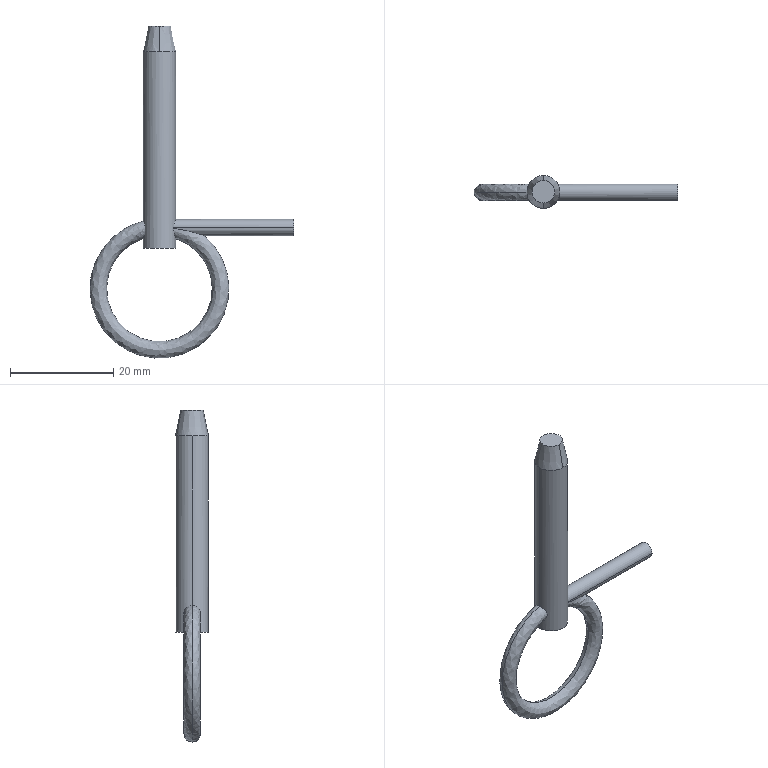Part | SolidWorks | features BaseBody 1 | 1 solid | 11 faces | box 39.425 x 6.35 x 64.25 mm | volume 2028 mm3 | cylinder 4 | plane 3 | cone 2 | spline 2 | commonest cylinder face diameters 3.2 x2 6.35 x2
STEP:
#1=CARTESIAN_POINT('',(3.175,0.,38.));
#2=VERTEX_POINT('',#1);
#3=CARTESIAN_POINT('',(0.,3.175,38.));
#4=VERTEX_POINT('',#3);
#5=CARTESIAN_POINT('',(0.,0.,38.));
#6=DIRECTION('',(0.,0.,1.));
#7=DIRECTION('',(-1.,0.,0.));
#8=AXIS2_PLACEMENT_3D('',#5,#6,#7);
#9=CIRCLE('',#8,3.175);
#10=EDGE_CURVE('',#2,#4,#9,.T.);
#11=ORIENTED_EDGE('',*,*,#10,.F.);
#12=CARTESIAN_POINT('',(3.175,0.,5.6));
#13=VERTEX_POINT('',#12);
#14=CARTESIAN_POINT('',(3.175,0.,38.));
#15=DIRECTION('',(0.,0.,-1.));
#16=VECTOR('',#15,1000.);
#17=LINE('',#14,#16);
#18=EDGE_CURVE('',#2,#13,#17,.T.);
#19=ORIENTED_EDGE('',*,*,#18,.T.);
#20=CARTESIAN_POINT('',(2.757,1.575,4.));
#21=VERTEX_POINT('',#20);
#22=CARTESIAN_POINT('',(2.757,1.575,4.));
#23=CARTESIAN_POINT('',(2.757,1.575,4.21));
#24=CARTESIAN_POINT('',(2.782,1.532,4.421));
#25=CARTESIAN_POINT('',(2.843,1.414,4.707));
#26=CARTESIAN_POINT('',(2.867,1.365,4.799));
#27=CARTESIAN_POINT('',(2.919,1.252,4.97));
#28=CARTESIAN_POINT('',(2.946,1.188,5.049));
#29=CARTESIAN_POINT('',(3.026,0.9722,5.268));
#30=CARTESIAN_POINT('',(3.078,0.8032,5.385));
#31=CARTESIAN_POINT('',(3.153,0.4186,5.551));
#32=CARTESIAN_POINT('',(3.175,0.2132,5.596));
#33=CARTESIAN_POINT('',(3.175,0.,5.6));
#34=B_SPLINE_CURVE_WITH_KNOTS('',3,(#22,#23,#24,#25,#26,#27,#28,#29,#30,#31,#32,#33),.UNSPECIFIED.,.F.,.F.,(4,2,2,2,2,4),(0.0001604,0.00079,0.001105,0.00142,0.002049,0.002679),.UNSPECIFIED.);
#35=EDGE_CURVE('',#21,#13,#34,.T.);
#36=ORIENTED_EDGE('',*,*,#35,.F.);
#37=CARTESIAN_POINT('',(2.761,1.567,3.839));
#38=VERTEX_POINT('',#37);
#39=CARTESIAN_POINT('',(2.761,1.567,3.839));
#40=CARTESIAN_POINT('',(2.758,1.572,3.893));
#41=CARTESIAN_POINT('',(2.757,1.575,3.946));
#42=CARTESIAN_POINT('',(2.757,1.575,4.));
#43=B_SPLINE_CURVE_WITH_KNOTS('',3,(#39,#40,#41,#42),.UNSPECIFIED.,.F.,.F.,(4,4),(0.,0.0001604),.UNSPECIFIED.);
#44=EDGE_CURVE('',#38,#21,#43,.T.);
#45=ORIENTED_EDGE('',*,*,#44,.F.);
#46=CARTESIAN_POINT('',(3.175,-0.000000001,1.895));
#47=VERTEX_POINT('',#46);
#48=CARTESIAN_POINT('',(3.175,-0.000000001,1.895));
#49=CARTESIAN_POINT('',(3.175,0.1189,1.897));
#50=CARTESIAN_POINT('',(3.168,0.2343,1.914));
#51=CARTESIAN_POINT('',(3.144,0.4588,1.979));
#52=CARTESIAN_POINT('',(3.126,0.5674,2.026));
#53=CARTESIAN_POINT('',(3.082,0.7678,2.14));
#54=CARTESIAN_POINT('',(3.057,0.8621,2.209));
#55=CARTESIAN_POINT('',(3.004,1.033,2.361));
#56=CARTESIAN_POINT('',(2.976,1.109,2.444));
#57=CARTESIAN_POINT('',(2.92,1.248,2.625));
#58=CARTESIAN_POINT('',(2.893,1.31,2.723));
#59=CARTESIAN_POINT('',(2.843,1.415,2.926));
#60=CARTESIAN_POINT('',(2.82,1.459,3.032));
#61=CARTESIAN_POINT('',(2.765,1.562,3.365));
#62=CARTESIAN_POINT('',(2.748,1.59,3.603));
#63=CARTESIAN_POINT('',(2.761,1.567,3.839));
#64=B_SPLINE_CURVE_WITH_KNOTS('',3,(#48,#49,#50,#51,#52,#53,#54,#55,#56,#57,#58,#59,#60,#61,#62,#63),.UNSPECIFIED.,.F.,.F.,(4,2,2,2,2,2,2,4),(0.,0.0003506,0.0007013,0.001052,0.001403,0.001753,0.002104,0.002805),.UNSPECIFIED.);
#65=EDGE_CURVE('',#47,#38,#64,.T.);
#66=ORIENTED_EDGE('',*,*,#65,.F.);
#67=CARTESIAN_POINT('',(3.175,0.,0.));
#68=VERTEX_POINT('',#67);
#69=CARTESIAN_POINT('',(3.175,0.,38.));
#70=DIRECTION('',(0.,0.,-1.));
#71=VECTOR('',#70,1000.);
#72=LINE('',#69,#71);
#73=EDGE_CURVE('',#47,#68,#72,.T.);
#74=ORIENTED_EDGE('',*,*,#73,.T.);
#75=CARTESIAN_POINT('',(-3.175,0.,0.));
#76=VERTEX_POINT('',#75);
#77=CARTESIAN_POINT('',(0.,0.,0.));
#78=DIRECTION('',(0.,0.,-1.));
#79=DIRECTION('',(-1.,0.,0.));
#80=AXIS2_PLACEMENT_3D('',#77,#78,#79);
#81=CIRCLE('',#80,3.175);
#82=EDGE_CURVE('',#76,#68,#81,.T.);
#83=ORIENTED_EDGE('',*,*,#82,.F.);
#84=CARTESIAN_POINT('',(-3.175,-0.000000001,1.895));
#85=VERTEX_POINT('',#84);
#86=CARTESIAN_POINT('',(-3.175,0.,38.));
#87=DIRECTION('',(0.,0.,-1.));
#88=VECTOR('',#87,1000.);
#89=LINE('',#86,#88);
#90=EDGE_CURVE('',#85,#76,#89,.T.);
#91=ORIENTED_EDGE('',*,*,#90,.F.);
#92=CARTESIAN_POINT('',(-3.175,-0.000000001,5.219));
#93=VERTEX_POINT('',#92);
#94=CARTESIAN_POINT('',(-3.175,-0.000000001,5.219));
#95=CARTESIAN_POINT('',(-3.175,0.1084,5.217));
#96=CARTESIAN_POINT('',(-3.169,0.2146,5.206));
#97=CARTESIAN_POINT('',(-3.148,0.4231,5.163));
#98=CARTESIAN_POINT('',(-3.133,0.5264,5.132));
#99=CARTESIAN_POINT('',(-3.093,0.7218,5.053));
#100=CARTESIAN_POINT('',(-3.07,0.8142,5.004));
#101=CARTESIAN_POINT('',(-3.019,0.9884,4.889));
#102=CARTESIAN_POINT('',(-2.99,1.07,4.823));
#103=CARTESIAN_POINT('',(-2.906,1.288,4.604));
#104=CARTESIAN_POINT('',(-2.849,1.404,4.424));
#105=CARTESIAN_POINT('',(-2.791,1.514,4.13));
#106=CARTESIAN_POINT('',(-2.776,1.541,4.025));
#107=CARTESIAN_POINT('',(-2.758,1.573,3.813));
#108=CARTESIAN_POINT('',(-2.755,1.578,3.707));
#109=CARTESIAN_POINT('',(-2.763,1.564,3.383));
#110=CARTESIAN_POINT('',(-2.792,1.514,3.172));
#111=CARTESIAN_POINT('',(-2.874,1.353,2.781));
#112=CARTESIAN_POINT('',(-2.926,1.241,2.601));
#113=CARTESIAN_POINT('',(-3.002,1.037,2.366));
#114=CARTESIAN_POINT('',(-3.027,0.9623,2.294));
#115=CARTESIAN_POINT('',(-3.074,0.7996,2.163));
#116=CARTESIAN_POINT('',(-3.096,0.7104,2.104));
#117=CARTESIAN_POINT('',(-3.152,0.4294,1.957));
#118=CARTESIAN_POINT('',(-3.175,0.2174,1.898));
#119=CARTESIAN_POINT('',(-3.175,-0.000000001,1.895));
#120=B_SPLINE_CURVE_WITH_KNOTS('',3,(#94,#95,#96,#97,#98,#99,#100,#101,#102,#103,#104,#105,#106,#107,#108,#109,#110,#111,#112,#113,#114,#115,#116,#117,#118,#119),.UNSPECIFIED.,.F.,.F.,(4,2,2,2,2,2,2,2,2,2,2,2,4),(0.,0.0003204,0.0006408,0.0009611,0.001282,0.001922,0.002243,0.002563,0.003204,0.003845,0.004165,0.004485,0.005126),.UNSPECIFIED.);
#121=EDGE_CURVE('',#93,#85,#120,.T.);
#122=ORIENTED_EDGE('',*,*,#121,.F.);
#123=CARTESIAN_POINT('',(-3.175,0.,38.));
#124=VERTEX_POINT('',#123);
#125=CARTESIAN_POINT('',(-3.175,0.,38.));
#126=DIRECTION('',(0.,0.,-1.));
#127=VECTOR('',#126,1000.);
#128=LINE('',#125,#127);
#129=EDGE_CURVE('',#124,#93,#128,.T.);
#130=ORIENTED_EDGE('',*,*,#129,.F.);
#131=CARTESIAN_POINT('',(0.,0.,38.));
#132=DIRECTION('',(0.,0.,1.));
#133=DIRECTION('',(-1.,0.,0.));
#134=AXIS2_PLACEMENT_3D('',#131,#132,#133);
#135=CIRCLE('',#134,3.175);
#136=EDGE_CURVE('',#4,#124,#135,.T.);
#137=ORIENTED_EDGE('',*,*,#136,.F.);
#138=EDGE_LOOP('',(#11,#19,#36,#45,#66,#74,#83,#91,#122,#130,#137));
#139=FACE_OUTER_BOUND('',#138,.T.);
#140=CARTESIAN_POINT('',(0.,0.,38.));
#141=DIRECTION('',(0.,0.,-1.));
#142=DIRECTION('',(-1.,0.,0.));
#143=AXIS2_PLACEMENT_3D('',#140,#141,#142);
#144=CYLINDRICAL_SURFACE('',#143,3.175);
#145=ADVANCED_FACE('',(#139),#144,.T.);
#146=CARTESIAN_POINT('',(26.,1.575,4.));
#147=VERTEX_POINT('',#146);
#148=CARTESIAN_POINT('',(26.,-1.625,4.));
#149=VERTEX_POINT('',#148);
#150=CARTESIAN_POINT('',(26.,-0.025,4.));
#151=DIRECTION('',(1.,0.,0.));
#152=DIRECTION('',(0.,-1.,0.));
#153=AXIS2_PLACEMENT_3D('',#150,#151,#152);
#154=CIRCLE('',#153,1.6);
#155=EDGE_CURVE('',#147,#149,#154,.T.);
#156=ORIENTED_EDGE('',*,*,#155,.F.);
#157=CARTESIAN_POINT('',(26.,1.575,4.));
#158=DIRECTION('',(-1.,0.,0.));
#159=VECTOR('',#158,1000.);
#160=LINE('',#157,#159);
#161=EDGE_CURVE('',#147,#21,#160,.T.);
#162=ORIENTED_EDGE('',*,*,#161,.T.);
#163=ORIENTED_EDGE('',*,*,#35,.T.);
#164=CARTESIAN_POINT('',(2.728,-1.625,4.));
#165=VERTEX_POINT('',#164);
#166=CARTESIAN_POINT('',(3.175,0.,5.6));
#167=CARTESIAN_POINT('',(3.175,-0.1089,5.601));
#168=CARTESIAN_POINT('',(3.169,-0.2161,5.592));
#169=CARTESIAN_POINT('',(3.148,-0.4259,5.553));
#170=CARTESIAN_POINT('',(3.132,-0.5298,5.522));
#171=CARTESIAN_POINT('',(3.073,-0.8242,5.402));
#172=CARTESIAN_POINT('',(3.017,-1.002,5.284));
#173=CARTESIAN_POINT('',(2.903,-1.296,4.993));
#174=CARTESIAN_POINT('',(2.843,-1.416,4.818));
#175=CARTESIAN_POINT('',(2.777,-1.539,4.528));
#176=CARTESIAN_POINT('',(2.759,-1.571,4.425));
#177=CARTESIAN_POINT('',(2.734,-1.614,4.215));
#178=CARTESIAN_POINT('',(2.728,-1.625,4.108));
#179=CARTESIAN_POINT('',(2.728,-1.625,4.));
#180=B_SPLINE_CURVE_WITH_KNOTS('',3,(#166,#167,#168,#169,#170,#171,#172,#173,#174,#175,#176,#177,#178,#179),.UNSPECIFIED.,.F.,.F.,(4,2,2,2,2,2,4),(0.002679,0.003,0.003322,0.003965,0.004608,0.00493,0.005251),.UNSPECIFIED.);
#181=EDGE_CURVE('',#13,#165,#180,.T.);
#182=ORIENTED_EDGE('',*,*,#181,.T.);
#183=CARTESIAN_POINT('',(26.,-1.625,4.));
#184=DIRECTION('',(-1.,0.,0.));
#185=VECTOR('',#184,1000.);
#186=LINE('',#183,#185);
#187=EDGE_CURVE('',#149,#165,#186,.T.);
#188=ORIENTED_EDGE('',*,*,#187,.F.);
#189=EDGE_LOOP('',(#156,#162,#163,#182,#188));
#190=FACE_OUTER_BOUND('',#189,.T.);
#191=CARTESIAN_POINT('',(26.,-0.025,4.));
#192=DIRECTION('',(-1.,0.,0.));
#193=DIRECTION('',(0.,-1.,0.));
#194=AXIS2_PLACEMENT_3D('',#191,#192,#193);
#195=CYLINDRICAL_SURFACE('',#194,1.6);
#196=ADVANCED_FACE('',(#190),#195,.T.);
#197=CARTESIAN_POINT('',(0.,-2.175,43.));
#198=VERTEX_POINT('',#197);
#199=CARTESIAN_POINT('',(0.,2.175,43.));
#200=VERTEX_POINT('',#199);
#201=CARTESIAN_POINT('',(0.,0.,43.));
#202=DIRECTION('',(0.,0.,1.));
#203=DIRECTION('',(0.,1.,0.));
#204=AXIS2_PLACEMENT_3D('',#201,#202,#203);
#205=CIRCLE('',#204,2.175);
#206=EDGE_CURVE('',#198,#200,#205,.T.);
#207=ORIENTED_EDGE('',*,*,#206,.F.);
#208=CARTESIAN_POINT('',(0.,-3.175,38.));
#209=VERTEX_POINT('',#208);
#210=CARTESIAN_POINT('',(0.,-2.175,43.));
#211=DIRECTION('',(0.,-0.1961,-0.9806));
#212=VECTOR('',#211,1000.);
#213=LINE('',#210,#212);
#214=EDGE_CURVE('',#198,#209,#213,.T.);
#215=ORIENTED_EDGE('',*,*,#214,.T.);
#216=CARTESIAN_POINT('',(0.,0.,38.));
#217=DIRECTION('',(0.,0.,1.));
#218=DIRECTION('',(-1.,0.,0.));
#219=AXIS2_PLACEMENT_3D('',#216,#217,#218);
#220=CIRCLE('',#219,3.175);
#221=EDGE_CURVE('',#209,#2,#220,.T.);
#222=ORIENTED_EDGE('',*,*,#221,.T.);
#223=ORIENTED_EDGE('',*,*,#10,.T.);
#224=CARTESIAN_POINT('',(0.,2.175,43.));
#225=DIRECTION('',(0.,0.1961,-0.9806));
#226=VECTOR('',#225,1000.);
#227=LINE('',#224,#226);
#228=EDGE_CURVE('',#200,#4,#227,.T.);
#229=ORIENTED_EDGE('',*,*,#228,.F.);
#230=EDGE_LOOP('',(#207,#215,#222,#223,#229));
#231=FACE_OUTER_BOUND('',#230,.T.);
#232=CARTESIAN_POINT('',(0.,0.,43.));
#233=DIRECTION('',(0.,0.,-1.));
#234=DIRECTION('',(0.,1.,0.));
#235=AXIS2_PLACEMENT_3D('',#232,#233,#234);
#236=CONICAL_SURFACE('',#235,2.175,0.1974);
#237=ADVANCED_FACE('',(#231),#236,.T.);
#238=CARTESIAN_POINT('',(-3.175,-0.025,1.895));
#239=VERTEX_POINT('',#238);
#240=CARTESIAN_POINT('',(3.175,-0.025,1.895));
#241=VERTEX_POINT('',#240);
#242=CARTESIAN_POINT('',(-0.000000001,-0.025,-7.825));
#243=DIRECTION('',(0.,-1.,0.));
#244=DIRECTION('',(1.,0.,0.));
#245=AXIS2_PLACEMENT_3D('',#242,#243,#244);
#246=CIRCLE('',#245,10.225);
#247=EDGE_CURVE('',#239,#241,#246,.T.);
#248=ORIENTED_EDGE('',*,*,#247,.T.);
#249=CARTESIAN_POINT('',(3.175,-0.025,1.895));
#250=CARTESIAN_POINT('',(3.175,-0.01667,1.894));
#251=CARTESIAN_POINT('',(3.175,-0.008333,1.895));
#252=CARTESIAN_POINT('',(3.175,-0.000000001,1.895));
#253=B_SPLINE_CURVE_WITH_KNOTS('',3,(#249,#250,#251,#252),.UNSPECIFIED.,.F.,.F.,(4,4),(-0.00002457,0.),.UNSPECIFIED.);
#254=EDGE_CURVE('',#241,#47,#253,.T.);
#255=ORIENTED_EDGE('',*,*,#254,.T.);
#256=ORIENTED_EDGE('',*,*,#65,.T.);
#257=CARTESIAN_POINT('',(8.699,-0.025,2.4));
#258=VERTEX_POINT('',#257);
#259=CARTESIAN_POINT('',(2.761,1.567,3.839));
#260=CARTESIAN_POINT('',(3.313,1.56,3.774));
#261=CARTESIAN_POINT('',(3.86,1.548,3.691));
#262=CARTESIAN_POINT('',(4.946,1.495,3.489));
#263=CARTESIAN_POINT('',(5.486,1.454,3.37));
#264=CARTESIAN_POINT('',(6.287,1.343,3.166));
#265=CARTESIAN_POINT('',(6.551,1.297,3.094));
#266=CARTESIAN_POINT('',(7.073,1.181,2.944));
#267=CARTESIAN_POINT('',(7.33,1.11,2.865));
#268=CARTESIAN_POINT('',(7.827,0.9241,2.706));
#269=CARTESIAN_POINT('',(8.072,0.8098,2.623));
#270=CARTESIAN_POINT('',(8.392,0.5678,2.511));
#271=CARTESIAN_POINT('',(8.491,0.4751,2.476));
#272=CARTESIAN_POINT('',(8.646,0.2501,2.419));
#273=CARTESIAN_POINT('',(8.699,0.116,2.4));
#274=CARTESIAN_POINT('',(8.699,-0.025,2.4));
#275=B_SPLINE_CURVE_WITH_KNOTS('',3,(#259,#260,#261,#262,#263,#264,#265,#266,#267,#268,#269,#270,#271,#272,#273,#274),.UNSPECIFIED.,.F.,.F.,(4,2,2,2,2,2,2,4),(0.,0.00166,0.003319,0.004149,0.004979,0.005809,0.006224,0.006639),.UNSPECIFIED.);
#276=EDGE_CURVE('',#38,#258,#275,.T.);
#277=ORIENTED_EDGE('',*,*,#276,.T.);
#278=CARTESIAN_POINT('',(-3.175,-0.025,5.219));
#279=VERTEX_POINT('',#278);
#280=CARTESIAN_POINT('',(8.699,-0.025,2.4));
#281=CARTESIAN_POINT('',(21.288,-0.025,-8.311));
#282=CARTESIAN_POINT('',(13.353,-0.025,-21.275));
#283=CARTESIAN_POINT('',(-0.0256,-0.025,-21.25));
#284=CARTESIAN_POINT('',(-21.177,-0.025,-21.21));
#285=CARTESIAN_POINT('',(-24.398,-0.025,0.05335));
#286=CARTESIAN_POINT('',(-3.175,-0.025,5.219));
#287=(BOUNDED_CURVE()B_SPLINE_CURVE(3,(#280,#281,#282,#283,#284,#285,#286),.UNSPECIFIED.,.F.,.F.)B_SPLINE_CURVE_WITH_KNOTS((4,3,4),(0.,0.4466,1.),.UNSPECIFIED.)CURVE()GEOMETRIC_REPRESENTATION_ITEM()RATIONAL_B_SPLINE_CURVE((0.6712,0.408,0.504,0.9594,0.3951,0.3826,0.9219))REPRESENTATION_ITEM(''));
#288=EDGE_CURVE('',#258,#279,#287,.T.);
#289=ORIENTED_EDGE('',*,*,#288,.T.);
#290=CARTESIAN_POINT('',(-3.175,-0.025,5.219));
#291=CARTESIAN_POINT('',(-3.175,-0.01667,5.219));
#292=CARTESIAN_POINT('',(-3.175,-0.008333,5.219));
#293=CARTESIAN_POINT('',(-3.175,-0.000000001,5.219));
#294=B_SPLINE_CURVE_WITH_KNOTS('',3,(#290,#291,#292,#293),.UNSPECIFIED.,.F.,.F.,(4,4),(-0.00002464,0.),.UNSPECIFIED.);
#295=EDGE_CURVE('',#279,#93,#294,.T.);
#296=ORIENTED_EDGE('',*,*,#295,.T.);
#297=ORIENTED_EDGE('',*,*,#121,.T.);
#298=CARTESIAN_POINT('',(-3.175,-0.000000001,1.895));
#299=CARTESIAN_POINT('',(-3.175,-0.008333,1.895));
#300=CARTESIAN_POINT('',(-3.175,-0.01667,1.894));
#301=CARTESIAN_POINT('',(-3.175,-0.025,1.895));
#302=B_SPLINE_CURVE_WITH_KNOTS('',3,(#298,#299,#300,#301),.UNSPECIFIED.,.F.,.F.,(4,4),(0.005126,0.005151),.UNSPECIFIED.);
#303=EDGE_CURVE('',#85,#239,#302,.T.);
#304=ORIENTED_EDGE('',*,*,#303,.T.);
#305=EDGE_LOOP('',(#248,#255,#256,#277,#289,#296,#297,#304));
#306=FACE_OUTER_BOUND('',#305,.T.);
#307=CARTESIAN_POINT('',(2.008,-0.1847,2.209));
#308=CARTESIAN_POINT('',(18.717,-0.1847,-1.135));
#309=CARTESIAN_POINT('',(17.02,-0.1847,-18.09));
#310=CARTESIAN_POINT('',(-0.01952,-0.1847,-18.058));
#311=CARTESIAN_POINT('',(-17.059,-0.1847,-18.025));
#312=CARTESIAN_POINT('',(-18.691,-0.1847,-1.064));
#313=CARTESIAN_POINT('',(-1.97,-0.1847,2.216));
#314=CARTESIAN_POINT('',(1.988,0.8235,2.11));
#315=CARTESIAN_POINT('',(18.532,0.8235,-1.201));
#316=CARTESIAN_POINT('',(16.852,0.8235,-17.989));
#317=CARTESIAN_POINT('',(-0.01932,0.8235,-17.957));
#318=CARTESIAN_POINT('',(-16.891,0.8235,-17.925));
#319=CARTESIAN_POINT('',(-18.506,0.8235,-1.131));
#320=CARTESIAN_POINT('',(-1.951,0.8235,2.117));
#321=CARTESIAN_POINT('',(2.122,1.575,2.776));
#322=CARTESIAN_POINT('',(19.775,1.575,-0.757));
#323=CARTESIAN_POINT('',(17.983,1.575,-18.671));
#324=CARTESIAN_POINT('',(-0.02062,1.575,-18.637));
#325=CARTESIAN_POINT('',(-18.024,1.575,-18.602));
#326=CARTESIAN_POINT('',(-19.748,1.575,-0.6816));
#327=CARTESIAN_POINT('',(-2.081,1.575,2.784));
#328=CARTESIAN_POINT('',(2.321,1.575,3.77));
#329=CARTESIAN_POINT('',(21.629,1.575,-0.09456));
#330=CARTESIAN_POINT('',(19.668,1.575,-19.687));
#331=CARTESIAN_POINT('',(-0.02255,1.575,-19.65));
#332=CARTESIAN_POINT('',(-19.713,1.575,-19.612));
#333=CARTESIAN_POINT('',(-21.599,1.575,-0.01212));
#334=CARTESIAN_POINT('',(-2.277,1.575,3.779));
#335=CARTESIAN_POINT('',(2.52,1.575,4.764));
#336=CARTESIAN_POINT('',(23.482,1.575,0.5679));
#337=CARTESIAN_POINT('',(21.354,1.575,-20.704));
#338=CARTESIAN_POINT('',(-0.02448,1.575,-20.663));
#339=CARTESIAN_POINT('',(-21.403,1.575,-20.622));
#340=CARTESIAN_POINT('',(-23.45,1.575,0.6574));
#341=CARTESIAN_POINT('',(-2.472,1.575,4.773));
#342=CARTESIAN_POINT('',(2.653,0.8235,5.43));
#343=CARTESIAN_POINT('',(24.725,0.8235,1.012));
#344=CARTESIAN_POINT('',(22.484,0.8235,-21.386));
#345=CARTESIAN_POINT('',(-0.02578,0.8235,-21.343));
#346=CARTESIAN_POINT('',(-22.536,0.8235,-21.3));
#347=CARTESIAN_POINT('',(-24.692,0.8235,1.107));
#348=CARTESIAN_POINT('',(-2.602,0.8235,5.44));
#349=CARTESIAN_POINT('',(2.633,-0.1847,5.331));
#350=CARTESIAN_POINT('',(24.54,-0.1847,0.9462));
#351=CARTESIAN_POINT('',(22.316,-0.1847,-21.285));
#352=CARTESIAN_POINT('',(-0.02559,-0.1847,-21.242));
#353=CARTESIAN_POINT('',(-22.367,-0.1847,-21.199));
#354=CARTESIAN_POINT('',(-24.507,-0.1847,1.04));
#355=CARTESIAN_POINT('',(-2.583,-0.1847,5.341));
#356=(BOUNDED_SURFACE()B_SPLINE_SURFACE(3,3,((#307,#308,#309,#310,#311,#312,#313),(#314,#315,#316,#317,#318,#319,#320),(#321,#322,#323,#324,#325,#326,#327),(#328,#329,#330,#331,#332,#333,#334),(#335,#336,#337,#338,#339,#340,#341),(#342,#343,#344,#345,#346,#347,#348),(#349,#350,#351,#352,#353,#354,#355)),.UNSPECIFIED.,.F.,.F.,.T.)B_SPLINE_SURFACE_WITH_KNOTS((4,3,4),(4,3,4),(0.,0.5,1.),(0.,0.5,1.),.UNSPECIFIED.)GEOMETRIC_REPRESENTATION_ITEM()RATIONAL_B_SPLINE_SURFACE(((1.,0.3984,0.3984,1.,0.3984,0.3984,1.),(0.7806,0.311,0.311,0.7806,0.311,0.311,0.7806),(0.7806,0.311,0.311,0.7806,0.311,0.311,0.7806),(1.,0.3984,0.3984,1.,0.3984,0.3984,1.),(0.7806,0.311,0.311,0.7806,0.311,0.311,0.7806),(0.7806,0.311,0.311,0.7806,0.311,0.311,0.7806),(1.,0.3984,0.3984,1.,0.3984,0.3984,1.)))REPRESENTATION_ITEM('')SURFACE());
#357=ADVANCED_FACE('',(#306),#356,.T.);
#358=ORIENTED_EDGE('',*,*,#18,.F.);
#359=ORIENTED_EDGE('',*,*,#221,.F.);
#360=CARTESIAN_POINT('',(0.,0.,38.));
#361=DIRECTION('',(0.,0.,1.));
#362=DIRECTION('',(-1.,0.,0.));
#363=AXIS2_PLACEMENT_3D('',#360,#361,#362);
#364=CIRCLE('',#363,3.175);
#365=EDGE_CURVE('',#124,#209,#364,.T.);
#366=ORIENTED_EDGE('',*,*,#365,.F.);
#367=ORIENTED_EDGE('',*,*,#129,.T.);
#368=ORIENTED_EDGE('',*,*,#295,.F.);
#369=CARTESIAN_POINT('',(-3.175,-0.025,1.895));
#370=CARTESIAN_POINT('',(-3.174,-0.1349,1.895));
#371=CARTESIAN_POINT('',(-3.168,-0.242,1.909));
#372=CARTESIAN_POINT('',(-3.145,-0.451,1.961));
#373=CARTESIAN_POINT('',(-3.128,-0.5533,2.));
#374=CARTESIAN_POINT('',(-3.068,-0.8384,2.145));
#375=CARTESIAN_POINT('',(-3.015,-1.006,2.281));
#376=CARTESIAN_POINT('',(-2.908,-1.283,2.595));
#377=CARTESIAN_POINT('',(-2.853,-1.397,2.777));
#378=CARTESIAN_POINT('',(-2.767,-1.561,3.167));
#379=CARTESIAN_POINT('',(-2.735,-1.612,3.381));
#380=CARTESIAN_POINT('',(-2.726,-1.628,3.706));
#381=CARTESIAN_POINT('',(-2.729,-1.623,3.817));
#382=CARTESIAN_POINT('',(-2.748,-1.591,4.03));
#383=CARTESIAN_POINT('',(-2.763,-1.565,4.134));
#384=CARTESIAN_POINT('',(-2.804,-1.489,4.335));
#385=CARTESIAN_POINT('',(-2.83,-1.441,4.429));
#386=CARTESIAN_POINT('',(-2.885,-1.327,4.606));
#387=CARTESIAN_POINT('',(-2.915,-1.26,4.688));
#388=CARTESIAN_POINT('',(-3.005,-1.038,4.908));
#389=CARTESIAN_POINT('',(-3.064,-0.8566,5.023));
#390=CARTESIAN_POINT('',(-3.127,-0.5601,5.14));
#391=CARTESIAN_POINT('',(-3.144,-0.4552,5.17));
#392=CARTESIAN_POINT('',(-3.168,-0.2426,5.209));
#393=CARTESIAN_POINT('',(-3.174,-0.1347,5.219));
#394=CARTESIAN_POINT('',(-3.175,-0.025,5.219));
#395=B_SPLINE_CURVE_WITH_KNOTS('',3,(#369,#370,#371,#372,#373,#374,#375,#376,#377,#378,#379,#380,#381,#382,#383,#384,#385,#386,#387,#388,#389,#390,#391,#392,#393,#394),.UNSPECIFIED.,.F.,.F.,(4,2,2,2,2,2,2,2,2,2,2,2,4),(0.,0.0003241,0.0006482,0.001296,0.001945,0.002593,0.002917,0.003241,0.003565,0.003889,0.004538,0.004862,0.005186),.UNSPECIFIED.);
#396=EDGE_CURVE('',#239,#279,#395,.T.);
#397=ORIENTED_EDGE('',*,*,#396,.F.);
#398=ORIENTED_EDGE('',*,*,#303,.F.);
#399=ORIENTED_EDGE('',*,*,#90,.T.);
#400=CARTESIAN_POINT('',(0.,0.,0.));
#401=DIRECTION('',(0.,0.,-1.));
#402=DIRECTION('',(-1.,0.,0.));
#403=AXIS2_PLACEMENT_3D('',#400,#401,#402);
#404=CIRCLE('',#403,3.175);
#405=EDGE_CURVE('',#68,#76,#404,.T.);
#406=ORIENTED_EDGE('',*,*,#405,.F.);
#407=ORIENTED_EDGE('',*,*,#73,.F.);
#408=ORIENTED_EDGE('',*,*,#254,.F.);
#409=CARTESIAN_POINT('',(2.732,-1.617,3.842));
#410=VERTEX_POINT('',#409);
#411=CARTESIAN_POINT('',(2.732,-1.617,3.842));
#412=CARTESIAN_POINT('',(2.725,-1.629,3.723));
#413=CARTESIAN_POINT('',(2.726,-1.627,3.605));
#414=CARTESIAN_POINT('',(2.742,-1.601,3.371));
#415=CARTESIAN_POINT('',(2.757,-1.576,3.253));
#416=CARTESIAN_POINT('',(2.815,-1.471,2.919));
#417=CARTESIAN_POINT('',(2.872,-1.361,2.711));
#418=CARTESIAN_POINT('',(2.99,-1.08,2.349));
#419=CARTESIAN_POINT('',(3.05,-0.9059,2.192));
#420=CARTESIAN_POINT('',(3.142,-0.4994,1.964));
#421=CARTESIAN_POINT('',(3.173,-0.2651,1.895));
#422=CARTESIAN_POINT('',(3.175,-0.025,1.895));
#423=B_SPLINE_CURVE_WITH_KNOTS('',3,(#411,#412,#413,#414,#415,#416,#417,#418,#419,#420,#421,#422),.UNSPECIFIED.,.F.,.F.,(4,2,2,2,2,4),(0.,0.0003537,0.0007075,0.001415,0.002122,0.00283),.UNSPECIFIED.);
#424=EDGE_CURVE('',#410,#241,#423,.T.);
#425=ORIENTED_EDGE('',*,*,#424,.F.);
#426=CARTESIAN_POINT('',(2.728,-1.625,4.));
#427=CARTESIAN_POINT('',(2.728,-1.625,3.947));
#428=CARTESIAN_POINT('',(2.729,-1.622,3.895));
#429=CARTESIAN_POINT('',(2.732,-1.617,3.842));
#430=B_SPLINE_CURVE_WITH_KNOTS('',3,(#426,#427,#428,#429),.UNSPECIFIED.,.F.,.F.,(4,4),(0.005251,0.005407),.UNSPECIFIED.);
#431=EDGE_CURVE('',#165,#410,#430,.T.);
#432=ORIENTED_EDGE('',*,*,#431,.F.);
#433=ORIENTED_EDGE('',*,*,#181,.F.);
#434=EDGE_LOOP('',(#358,#359,#366,#367,#368,#397,#398,#399,#406,#407,#408,#425,#432,#433));
#435=FACE_OUTER_BOUND('',#434,.T.);
#436=CARTESIAN_POINT('',(0.,0.,38.));
#437=DIRECTION('',(0.,0.,-1.));
#438=DIRECTION('',(-1.,0.,0.));
#439=AXIS2_PLACEMENT_3D('',#436,#437,#438);
#440=CYLINDRICAL_SURFACE('',#439,3.175);
#441=ADVANCED_FACE('',(#435),#440,.T.);
#442=ORIENTED_EDGE('',*,*,#247,.F.);
#443=ORIENTED_EDGE('',*,*,#396,.T.);
#444=ORIENTED_EDGE('',*,*,#288,.F.);
#445=CARTESIAN_POINT('',(8.699,-0.025,2.4));
#446=CARTESIAN_POINT('',(8.699,-0.168,2.4));
#447=CARTESIAN_POINT('',(8.645,-0.3029,2.42));
#448=CARTESIAN_POINT('',(8.487,-0.5301,2.477));
#449=CARTESIAN_POINT('',(8.386,-0.6233,2.513));
#450=CARTESIAN_POINT('',(8.168,-0.7858,2.59));
#451=CARTESIAN_POINT('',(8.052,-0.8539,2.629));
#452=CARTESIAN_POINT('',(7.814,-0.9735,2.709));
#453=CARTESIAN_POINT('',(7.691,-1.025,2.75));
#454=CARTESIAN_POINT('',(7.315,-1.164,2.87));
#455=CARTESIAN_POINT('',(7.055,-1.235,2.949));
#456=CARTESIAN_POINT('',(6.532,-1.351,3.099));
#457=CARTESIAN_POINT('',(6.268,-1.396,3.171));
#458=CARTESIAN_POINT('',(5.47,-1.505,3.373));
#459=CARTESIAN_POINT('',(4.93,-1.546,3.492));
#460=CARTESIAN_POINT('',(3.836,-1.599,3.695));
#461=CARTESIAN_POINT('',(3.285,-1.611,3.778));
#462=CARTESIAN_POINT('',(2.732,-1.617,3.842));
#463=B_SPLINE_CURVE_WITH_KNOTS('',3,(#445,#446,#447,#448,#449,#450,#451,#452,#453,#454,#455,#456,#457,#458,#459,#460,#461,#462),.UNSPECIFIED.,.F.,.F.,(4,2,2,2,2,2,2,2,4),(0.,0.0004218,0.0008436,0.001265,0.001687,0.002531,0.003374,0.005062,0.006749),.UNSPECIFIED.);
#464=EDGE_CURVE('',#258,#410,#463,.T.);
#465=ORIENTED_EDGE('',*,*,#464,.T.);
#466=ORIENTED_EDGE('',*,*,#424,.T.);
#467=EDGE_LOOP('',(#442,#443,#444,#465,#466));
#468=FACE_OUTER_BOUND('',#467,.T.);
#469=CARTESIAN_POINT('',(2.601,0.1347,5.337));
#470=CARTESIAN_POINT('',(24.564,0.1347,0.9977));
#471=CARTESIAN_POINT('',(22.364,0.1347,-21.282));
#472=CARTESIAN_POINT('',(-0.02387,0.1347,-21.242));
#473=CARTESIAN_POINT('',(-22.412,0.1347,-21.202));
#474=CARTESIAN_POINT('',(-24.532,0.1347,1.085));
#475=CARTESIAN_POINT('',(-2.554,0.1347,5.347));
#476=CARTESIAN_POINT('',(2.62,-0.8735,5.437));
#477=CARTESIAN_POINT('',(24.749,-0.8735,1.064));
#478=CARTESIAN_POINT('',(22.532,-0.8735,-21.383));
#479=CARTESIAN_POINT('',(-0.02405,-0.8735,-21.343));
#480=CARTESIAN_POINT('',(-22.581,-0.8735,-21.303));
#481=CARTESIAN_POINT('',(-24.717,-0.8735,1.152));
#482=CARTESIAN_POINT('',(-2.573,-0.8735,5.446));
#483=CARTESIAN_POINT('',(2.489,-1.625,4.77));
#484=CARTESIAN_POINT('',(23.505,-1.625,0.6172));
#485=CARTESIAN_POINT('',(21.399,-1.625,-20.701));
#486=CARTESIAN_POINT('',(-0.02284,-1.625,-20.663));
#487=CARTESIAN_POINT('',(-21.445,-1.625,-20.625));
#488=CARTESIAN_POINT('',(-23.474,-1.625,0.7007));
#489=CARTESIAN_POINT('',(-2.444,-1.625,4.779));
#490=CARTESIAN_POINT('',(2.292,-1.625,3.776));
#491=CARTESIAN_POINT('',(21.649,-1.625,-0.0492));
#492=CARTESIAN_POINT('',(19.71,-1.625,-19.685));
#493=CARTESIAN_POINT('',(-0.02104,-1.625,-19.65));
#494=CARTESIAN_POINT('',(-19.752,-1.625,-19.615));
#495=CARTESIAN_POINT('',(-21.621,-1.625,0.02779));
#496=CARTESIAN_POINT('',(-2.251,-1.625,3.784));
#497=CARTESIAN_POINT('',(2.096,-1.625,2.782));
#498=CARTESIAN_POINT('',(19.794,-1.625,-0.7155));
#499=CARTESIAN_POINT('',(18.021,-1.625,-18.669));
#500=CARTESIAN_POINT('',(-0.01924,-1.625,-18.637));
#501=CARTESIAN_POINT('',(-18.06,-1.625,-18.604));
#502=CARTESIAN_POINT('',(-19.769,-1.625,-0.6452));
#503=CARTESIAN_POINT('',(-2.058,-1.625,2.789));
#504=CARTESIAN_POINT('',(1.964,-0.8735,2.115));
#505=CARTESIAN_POINT('',(18.549,-0.8735,-1.163));
#506=CARTESIAN_POINT('',(16.888,-0.8735,-17.987));
#507=CARTESIAN_POINT('',(-0.01803,-0.8735,-17.957));
#508=CARTESIAN_POINT('',(-16.924,-0.8735,-17.927));
#509=CARTESIAN_POINT('',(-18.526,-0.8735,-1.097));
#510=CARTESIAN_POINT('',(-1.929,-0.8735,2.121));
#511=CARTESIAN_POINT('',(1.984,0.1347,2.214));
#512=CARTESIAN_POINT('',(18.735,0.1347,-1.096));
#513=CARTESIAN_POINT('',(17.057,0.1347,-18.088));
#514=CARTESIAN_POINT('',(-0.01821,0.1347,-18.058));
#515=CARTESIAN_POINT('',(-17.093,0.1347,-18.028));
#516=CARTESIAN_POINT('',(-18.711,0.1347,-1.029));
#517=CARTESIAN_POINT('',(-1.948,0.1347,2.221));
#518=(BOUNDED_SURFACE()B_SPLINE_SURFACE(3,3,((#469,#470,#471,#472,#473,#474,#475),(#476,#477,#478,#479,#480,#481,#482),(#483,#484,#485,#486,#487,#488,#489),(#490,#491,#492,#493,#494,#495,#496),(#497,#498,#499,#500,#501,#502,#503),(#504,#505,#506,#507,#508,#509,#510),(#511,#512,#513,#514,#515,#516,#517)),.UNSPECIFIED.,.F.,.F.,.T.)B_SPLINE_SURFACE_WITH_KNOTS((4,3,4),(4,3,4),(0.,0.5,1.),(0.,0.5,1.),.UNSPECIFIED.)GEOMETRIC_REPRESENTATION_ITEM()RATIONAL_B_SPLINE_SURFACE(((1.,0.3977,0.3977,1.,0.3977,0.3977,1.),(0.7806,0.3104,0.3104,0.7806,0.3104,0.3104,0.7806),(0.7806,0.3104,0.3104,0.7806,0.3104,0.3104,0.7806),(1.,0.3977,0.3977,1.,0.3977,0.3977,1.),(0.7806,0.3104,0.3104,0.7806,0.3104,0.3104,0.7806),(0.7806,0.3104,0.3104,0.7806,0.3104,0.3104,0.7806),(1.,0.3977,0.3977,1.,0.3977,0.3977,1.)))REPRESENTATION_ITEM('')SURFACE());
#519=ADVANCED_FACE('',(#468),#518,.T.);
#520=ORIENTED_EDGE('',*,*,#161,.F.);
#521=CARTESIAN_POINT('',(26.,-0.025,4.));
#522=DIRECTION('',(1.,0.,0.));
#523=DIRECTION('',(0.,-1.,0.));
#524=AXIS2_PLACEMENT_3D('',#521,#522,#523);
#525=CIRCLE('',#524,1.6);
#526=EDGE_CURVE('',#149,#147,#525,.T.);
#527=ORIENTED_EDGE('',*,*,#526,.F.);
#528=ORIENTED_EDGE('',*,*,#187,.T.);
#529=ORIENTED_EDGE('',*,*,#431,.T.);
#530=ORIENTED_EDGE('',*,*,#464,.F.);
#531=ORIENTED_EDGE('',*,*,#276,.F.);
#532=ORIENTED_EDGE('',*,*,#44,.T.);
#533=EDGE_LOOP('',(#520,#527,#528,#529,#530,#531,#532));
#534=FACE_OUTER_BOUND('',#533,.T.);
#535=CARTESIAN_POINT('',(26.,-0.025,4.));
#536=DIRECTION('',(-1.,0.,0.));
#537=DIRECTION('',(0.,-1.,0.));
#538=AXIS2_PLACEMENT_3D('',#535,#536,#537);
#539=CYLINDRICAL_SURFACE('',#538,1.6);
#540=ADVANCED_FACE('',(#534),#539,.T.);
#541=ORIENTED_EDGE('',*,*,#214,.F.);
#542=CARTESIAN_POINT('',(0.,0.,43.));
#543=DIRECTION('',(0.,0.,1.));
#544=DIRECTION('',(0.,1.,0.));
#545=AXIS2_PLACEMENT_3D('',#542,#543,#544);
#546=CIRCLE('',#545,2.175);
#547=EDGE_CURVE('',#200,#198,#546,.T.);
#548=ORIENTED_EDGE('',*,*,#547,.F.);
#549=ORIENTED_EDGE('',*,*,#228,.T.);
#550=ORIENTED_EDGE('',*,*,#136,.T.);
#551=ORIENTED_EDGE('',*,*,#365,.T.);
#552=EDGE_LOOP('',(#541,#548,#549,#550,#551));
#553=FACE_OUTER_BOUND('',#552,.T.);
#554=CARTESIAN_POINT('',(0.,0.,43.));
#555=DIRECTION('',(0.,0.,-1.));
#556=DIRECTION('',(0.,1.,0.));
#557=AXIS2_PLACEMENT_3D('',#554,#555,#556);
#558=CONICAL_SURFACE('',#557,2.175,0.1974);
#559=ADVANCED_FACE('',(#553),#558,.T.);
#560=ORIENTED_EDGE('',*,*,#82,.T.);
#561=ORIENTED_EDGE('',*,*,#405,.T.);
#562=EDGE_LOOP('',(#560,#561));
#563=FACE_OUTER_BOUND('',#562,.T.);
#564=CARTESIAN_POINT('',(-3.213,-3.213,0.));
#565=DIRECTION('',(0.,0.,1.));
#566=DIRECTION('',(1.,0.,0.));
#567=AXIS2_PLACEMENT_3D('',#564,#565,#566);
#568=PLANE('',#567);
#569=ADVANCED_FACE('',(#563),#568,.F.);
#570=ORIENTED_EDGE('',*,*,#526,.T.);
#571=ORIENTED_EDGE('',*,*,#155,.T.);
#572=EDGE_LOOP('',(#570,#571));
#573=FACE_OUTER_BOUND('',#572,.T.);
#574=CARTESIAN_POINT('',(26.,-1.644,5.619));
#575=DIRECTION('',(1.,0.,0.));
#576=DIRECTION('',(0.,0.,-1.));
#577=AXIS2_PLACEMENT_3D('',#574,#575,#576);
#578=PLANE('',#577);
#579=ADVANCED_FACE('',(#573),#578,.T.);
#580=ORIENTED_EDGE('',*,*,#547,.T.);
#581=ORIENTED_EDGE('',*,*,#206,.T.);
#582=EDGE_LOOP('',(#580,#581));
#583=FACE_OUTER_BOUND('',#582,.T.);
#584=CARTESIAN_POINT('',(-2.201,-2.201,43.));
#585=DIRECTION('',(0.,0.,1.));
#586=DIRECTION('',(1.,0.,0.));
#587=AXIS2_PLACEMENT_3D('',#584,#585,#586);
#588=PLANE('',#587);
#589=ADVANCED_FACE('',(#583),#588,.T.);
#590=CLOSED_SHELL('',(#145,#196,#237,#357,#441,#519,#540,#559,#569,#579,#589));
#591=MANIFOLD_SOLID_BREP('',#590);
#592=CARTESIAN_POINT('',(0.,0.,0.));
#593=DIRECTION('',(0.,0.,1.));
#594=DIRECTION('',(1.,0.,0.));
#595=AXIS2_PLACEMENT_3D('',#592,#593,#594);
#596=(LENGTH_UNIT()NAMED_UNIT(*)SI_UNIT(.MILLI.,.METRE.));
#597=UNCERTAINTY_MEASURE_WITH_UNIT(LENGTH_MEASURE(0.00001),#596,'','');
#598=(NAMED_UNIT(*)PLANE_ANGLE_UNIT()SI_UNIT($,.RADIAN.));
#599=(NAMED_UNIT(*)SI_UNIT($,.STERADIAN.)SOLID_ANGLE_UNIT());
#600=(GEOMETRIC_REPRESENTATION_CONTEXT(3)GLOBAL_UNCERTAINTY_ASSIGNED_CONTEXT((#597))GLOBAL_UNIT_ASSIGNED_CONTEXT((#596,#598,#599))REPRESENTATION_CONTEXT('',''));
#601=ADVANCED_BREP_SHAPE_REPRESENTATION('',(#591,#595),#600);